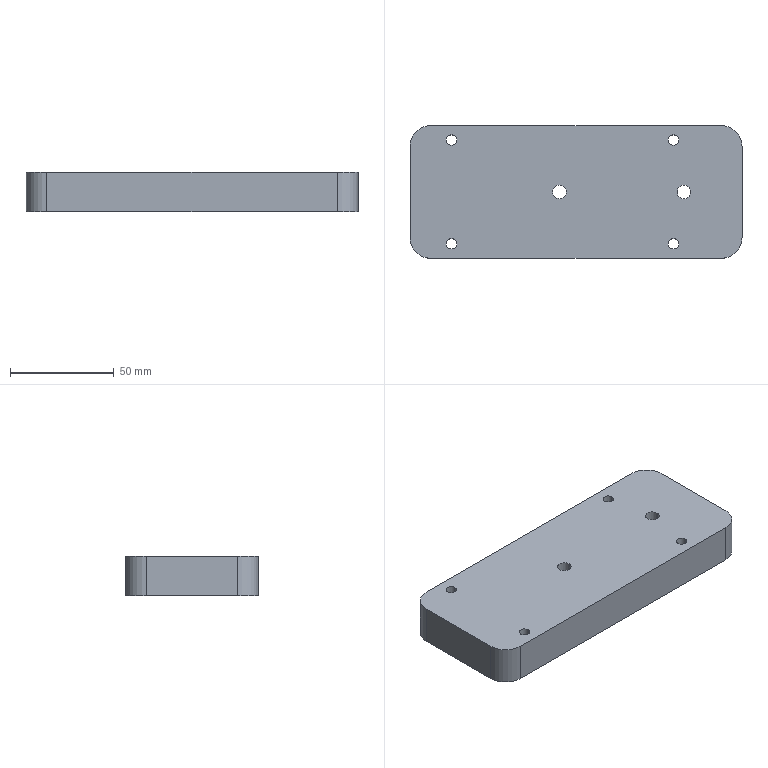Part | SolidWorks | features HoleWzd 2, Extrusion 1, Fillet 1 | 1 solid | 26 faces | box 160 x 64 x 19 mm | volume 189875 mm3 | cylinder 16 | plane 6 | cone 4 | commonest cylinder face diameters 5 x8 6.6 x4 20 x4
STEP:
#1=CARTESIAN_POINT('',(55.3,0.,3.1));
#2=VERTEX_POINT('',#1);
#3=CARTESIAN_POINT('',(48.7,0.,3.1));
#4=VERTEX_POINT('',#3);
#5=CARTESIAN_POINT('',(52.,0.,3.1));
#6=DIRECTION('',(0.,0.,-1.));
#7=DIRECTION('',(-1.,0.,0.));
#8=AXIS2_PLACEMENT_3D('',#5,#6,#7);
#9=CIRCLE('',#8,3.3);
#10=EDGE_CURVE('',#2,#4,#9,.T.);
#11=ORIENTED_EDGE('',*,*,#10,.F.);
#12=CARTESIAN_POINT('',(58.4,0.,0.));
#13=VERTEX_POINT('',#12);
#14=CARTESIAN_POINT('',(58.4,0.,0.));
#15=DIRECTION('',(0.7071,0.,-0.7071));
#16=VECTOR('',#15,1000.);
#17=LINE('',#14,#16);
#18=EDGE_CURVE('',#2,#13,#17,.T.);
#19=ORIENTED_EDGE('',*,*,#18,.T.);
#20=CARTESIAN_POINT('',(45.6,0.,0.));
#21=VERTEX_POINT('',#20);
#22=CARTESIAN_POINT('',(52.,0.,0.));
#23=DIRECTION('',(0.,0.,-1.));
#24=DIRECTION('',(-1.,0.,0.));
#25=AXIS2_PLACEMENT_3D('',#22,#23,#24);
#26=CIRCLE('',#25,6.4);
#27=EDGE_CURVE('',#13,#21,#26,.T.);
#28=ORIENTED_EDGE('',*,*,#27,.T.);
#29=CARTESIAN_POINT('',(45.6,0.,0.));
#30=DIRECTION('',(-0.7071,0.,-0.7071));
#31=VECTOR('',#30,1000.);
#32=LINE('',#29,#31);
#33=EDGE_CURVE('',#4,#21,#32,.T.);
#34=ORIENTED_EDGE('',*,*,#33,.F.);
#35=EDGE_LOOP('',(#11,#19,#28,#34));
#36=FACE_OUTER_BOUND('',#35,.T.);
#37=CARTESIAN_POINT('',(52.,0.,0.));
#38=DIRECTION('',(0.,0.,-1.));
#39=DIRECTION('',(-1.,0.,0.));
#40=AXIS2_PLACEMENT_3D('',#37,#38,#39);
#41=CONICAL_SURFACE('',#40,6.4,0.7854);
#42=ADVANCED_FACE('',(#36),#41,.F.);
#43=CARTESIAN_POINT('',(55.3,0.,19.));
#44=VERTEX_POINT('',#43);
#45=CARTESIAN_POINT('',(48.7,0.,19.));
#46=VERTEX_POINT('',#45);
#47=CARTESIAN_POINT('',(52.,0.,19.));
#48=DIRECTION('',(0.,0.,-1.));
#49=DIRECTION('',(-1.,0.,0.));
#50=AXIS2_PLACEMENT_3D('',#47,#48,#49);
#51=CIRCLE('',#50,3.3);
#52=EDGE_CURVE('',#44,#46,#51,.T.);
#53=ORIENTED_EDGE('',*,*,#52,.F.);
#54=CARTESIAN_POINT('',(55.3,0.,0.));
#55=DIRECTION('',(0.,0.,-1.));
#56=VECTOR('',#55,1000.);
#57=LINE('',#54,#56);
#58=EDGE_CURVE('',#44,#2,#57,.T.);
#59=ORIENTED_EDGE('',*,*,#58,.T.);
#60=ORIENTED_EDGE('',*,*,#10,.T.);
#61=CARTESIAN_POINT('',(48.7,0.,0.));
#62=DIRECTION('',(0.,0.,-1.));
#63=VECTOR('',#62,1000.);
#64=LINE('',#61,#63);
#65=EDGE_CURVE('',#46,#4,#64,.T.);
#66=ORIENTED_EDGE('',*,*,#65,.F.);
#67=EDGE_LOOP('',(#53,#59,#60,#66));
#68=FACE_OUTER_BOUND('',#67,.T.);
#69=CARTESIAN_POINT('',(52.,0.,0.));
#70=DIRECTION('',(0.,0.,-1.));
#71=DIRECTION('',(-1.,0.,0.));
#72=AXIS2_PLACEMENT_3D('',#69,#70,#71);
#73=CYLINDRICAL_SURFACE('',#72,3.3);
#74=ADVANCED_FACE('',(#68),#73,.F.);
#75=CARTESIAN_POINT('',(-4.7,0.,3.1));
#76=VERTEX_POINT('',#75);
#77=CARTESIAN_POINT('',(-11.3,0.,3.1));
#78=VERTEX_POINT('',#77);
#79=CARTESIAN_POINT('',(-8.,0.,3.1));
#80=DIRECTION('',(0.,0.,-1.));
#81=DIRECTION('',(-1.,0.,0.));
#82=AXIS2_PLACEMENT_3D('',#79,#80,#81);
#83=CIRCLE('',#82,3.3);
#84=EDGE_CURVE('',#76,#78,#83,.T.);
#85=ORIENTED_EDGE('',*,*,#84,.F.);
#86=CARTESIAN_POINT('',(-1.6,0.,0.));
#87=VERTEX_POINT('',#86);
#88=CARTESIAN_POINT('',(-1.6,0.,0.));
#89=DIRECTION('',(0.7071,0.,-0.7071));
#90=VECTOR('',#89,1000.);
#91=LINE('',#88,#90);
#92=EDGE_CURVE('',#76,#87,#91,.T.);
#93=ORIENTED_EDGE('',*,*,#92,.T.);
#94=CARTESIAN_POINT('',(-14.4,0.,0.));
#95=VERTEX_POINT('',#94);
#96=CARTESIAN_POINT('',(-8.,0.,0.));
#97=DIRECTION('',(0.,0.,-1.));
#98=DIRECTION('',(-1.,0.,0.));
#99=AXIS2_PLACEMENT_3D('',#96,#97,#98);
#100=CIRCLE('',#99,6.4);
#101=EDGE_CURVE('',#87,#95,#100,.T.);
#102=ORIENTED_EDGE('',*,*,#101,.T.);
#103=CARTESIAN_POINT('',(-14.4,0.,0.));
#104=DIRECTION('',(-0.7071,0.,-0.7071));
#105=VECTOR('',#104,1000.);
#106=LINE('',#103,#105);
#107=EDGE_CURVE('',#78,#95,#106,.T.);
#108=ORIENTED_EDGE('',*,*,#107,.F.);
#109=EDGE_LOOP('',(#85,#93,#102,#108));
#110=FACE_OUTER_BOUND('',#109,.T.);
#111=CARTESIAN_POINT('',(-8.,0.,0.));
#112=DIRECTION('',(0.,0.,-1.));
#113=DIRECTION('',(-1.,0.,0.));
#114=AXIS2_PLACEMENT_3D('',#111,#112,#113);
#115=CONICAL_SURFACE('',#114,6.4,0.7854);
#116=ADVANCED_FACE('',(#110),#115,.F.);
#117=CARTESIAN_POINT('',(-4.7,0.,19.));
#118=VERTEX_POINT('',#117);
#119=CARTESIAN_POINT('',(-11.3,0.,19.));
#120=VERTEX_POINT('',#119);
#121=CARTESIAN_POINT('',(-8.,0.,19.));
#122=DIRECTION('',(0.,0.,-1.));
#123=DIRECTION('',(-1.,0.,0.));
#124=AXIS2_PLACEMENT_3D('',#121,#122,#123);
#125=CIRCLE('',#124,3.3);
#126=EDGE_CURVE('',#118,#120,#125,.T.);
#127=ORIENTED_EDGE('',*,*,#126,.F.);
#128=CARTESIAN_POINT('',(-4.7,0.,0.));
#129=DIRECTION('',(0.,0.,-1.));
#130=VECTOR('',#129,1000.);
#131=LINE('',#128,#130);
#132=EDGE_CURVE('',#118,#76,#131,.T.);
#133=ORIENTED_EDGE('',*,*,#132,.T.);
#134=ORIENTED_EDGE('',*,*,#84,.T.);
#135=CARTESIAN_POINT('',(-11.3,0.,0.));
#136=DIRECTION('',(0.,0.,-1.));
#137=VECTOR('',#136,1000.);
#138=LINE('',#135,#137);
#139=EDGE_CURVE('',#120,#78,#138,.T.);
#140=ORIENTED_EDGE('',*,*,#139,.F.);
#141=EDGE_LOOP('',(#127,#133,#134,#140));
#142=FACE_OUTER_BOUND('',#141,.T.);
#143=CARTESIAN_POINT('',(-8.,0.,0.));
#144=DIRECTION('',(0.,0.,-1.));
#145=DIRECTION('',(-1.,0.,0.));
#146=AXIS2_PLACEMENT_3D('',#143,#144,#145);
#147=CYLINDRICAL_SURFACE('',#146,3.3);
#148=ADVANCED_FACE('',(#142),#147,.F.);
#149=CARTESIAN_POINT('',(-62.5,25.,0.));
#150=VERTEX_POINT('',#149);
#151=CARTESIAN_POINT('',(-57.5,25.,0.));
#152=VERTEX_POINT('',#151);
#153=CARTESIAN_POINT('',(-60.,25.,0.));
#154=DIRECTION('',(0.,0.,1.));
#155=DIRECTION('',(1.,0.,0.));
#156=AXIS2_PLACEMENT_3D('',#153,#154,#155);
#157=CIRCLE('',#156,2.5);
#158=EDGE_CURVE('',#150,#152,#157,.T.);
#159=ORIENTED_EDGE('',*,*,#158,.F.);
#160=CARTESIAN_POINT('',(-62.5,25.,19.));
#161=VERTEX_POINT('',#160);
#162=CARTESIAN_POINT('',(-62.5,25.,19.));
#163=DIRECTION('',(0.,0.,1.));
#164=VECTOR('',#163,1000.);
#165=LINE('',#162,#164);
#166=EDGE_CURVE('',#150,#161,#165,.T.);
#167=ORIENTED_EDGE('',*,*,#166,.T.);
#168=CARTESIAN_POINT('',(-57.5,25.,19.));
#169=VERTEX_POINT('',#168);
#170=CARTESIAN_POINT('',(-60.,25.,19.));
#171=DIRECTION('',(0.,0.,1.));
#172=DIRECTION('',(1.,0.,0.));
#173=AXIS2_PLACEMENT_3D('',#170,#171,#172);
#174=CIRCLE('',#173,2.5);
#175=EDGE_CURVE('',#161,#169,#174,.T.);
#176=ORIENTED_EDGE('',*,*,#175,.T.);
#177=CARTESIAN_POINT('',(-57.5,25.,19.));
#178=DIRECTION('',(0.,0.,1.));
#179=VECTOR('',#178,1000.);
#180=LINE('',#177,#179);
#181=EDGE_CURVE('',#152,#169,#180,.T.);
#182=ORIENTED_EDGE('',*,*,#181,.F.);
#183=EDGE_LOOP('',(#159,#167,#176,#182));
#184=FACE_OUTER_BOUND('',#183,.T.);
#185=CARTESIAN_POINT('',(-60.,25.,19.));
#186=DIRECTION('',(0.,0.,1.));
#187=DIRECTION('',(1.,0.,0.));
#188=AXIS2_PLACEMENT_3D('',#185,#186,#187);
#189=CYLINDRICAL_SURFACE('',#188,2.5);
#190=ADVANCED_FACE('',(#184),#189,.F.);
#191=CARTESIAN_POINT('',(-62.5,-25.,0.));
#192=VERTEX_POINT('',#191);
#193=CARTESIAN_POINT('',(-57.5,-25.,0.));
#194=VERTEX_POINT('',#193);
#195=CARTESIAN_POINT('',(-60.,-25.,0.));
#196=DIRECTION('',(0.,0.,1.));
#197=DIRECTION('',(1.,0.,0.));
#198=AXIS2_PLACEMENT_3D('',#195,#196,#197);
#199=CIRCLE('',#198,2.5);
#200=EDGE_CURVE('',#192,#194,#199,.T.);
#201=ORIENTED_EDGE('',*,*,#200,.F.);
#202=CARTESIAN_POINT('',(-62.5,-25.,19.));
#203=VERTEX_POINT('',#202);
#204=CARTESIAN_POINT('',(-62.5,-25.,19.));
#205=DIRECTION('',(0.,0.,1.));
#206=VECTOR('',#205,1000.);
#207=LINE('',#204,#206);
#208=EDGE_CURVE('',#192,#203,#207,.T.);
#209=ORIENTED_EDGE('',*,*,#208,.T.);
#210=CARTESIAN_POINT('',(-57.5,-25.,19.));
#211=VERTEX_POINT('',#210);
#212=CARTESIAN_POINT('',(-60.,-25.,19.));
#213=DIRECTION('',(0.,0.,1.));
#214=DIRECTION('',(1.,0.,0.));
#215=AXIS2_PLACEMENT_3D('',#212,#213,#214);
#216=CIRCLE('',#215,2.5);
#217=EDGE_CURVE('',#203,#211,#216,.T.);
#218=ORIENTED_EDGE('',*,*,#217,.T.);
#219=CARTESIAN_POINT('',(-57.5,-25.,19.));
#220=DIRECTION('',(0.,0.,1.));
#221=VECTOR('',#220,1000.);
#222=LINE('',#219,#221);
#223=EDGE_CURVE('',#194,#211,#222,.T.);
#224=ORIENTED_EDGE('',*,*,#223,.F.);
#225=EDGE_LOOP('',(#201,#209,#218,#224));
#226=FACE_OUTER_BOUND('',#225,.T.);
#227=CARTESIAN_POINT('',(-60.,-25.,19.));
#228=DIRECTION('',(0.,0.,1.));
#229=DIRECTION('',(1.,0.,0.));
#230=AXIS2_PLACEMENT_3D('',#227,#228,#229);
#231=CYLINDRICAL_SURFACE('',#230,2.5);
#232=ADVANCED_FACE('',(#226),#231,.F.);
#233=CARTESIAN_POINT('',(44.5,25.,0.));
#234=VERTEX_POINT('',#233);
#235=CARTESIAN_POINT('',(49.5,25.,0.));
#236=VERTEX_POINT('',#235);
#237=CARTESIAN_POINT('',(47.,25.,0.));
#238=DIRECTION('',(0.,0.,1.));
#239=DIRECTION('',(1.,0.,0.));
#240=AXIS2_PLACEMENT_3D('',#237,#238,#239);
#241=CIRCLE('',#240,2.5);
#242=EDGE_CURVE('',#234,#236,#241,.T.);
#243=ORIENTED_EDGE('',*,*,#242,.F.);
#244=CARTESIAN_POINT('',(44.5,25.,19.));
#245=VERTEX_POINT('',#244);
#246=CARTESIAN_POINT('',(44.5,25.,19.));
#247=DIRECTION('',(0.,0.,1.));
#248=VECTOR('',#247,1000.);
#249=LINE('',#246,#248);
#250=EDGE_CURVE('',#234,#245,#249,.T.);
#251=ORIENTED_EDGE('',*,*,#250,.T.);
#252=CARTESIAN_POINT('',(49.5,25.,19.));
#253=VERTEX_POINT('',#252);
#254=CARTESIAN_POINT('',(47.,25.,19.));
#255=DIRECTION('',(0.,0.,1.));
#256=DIRECTION('',(1.,0.,0.));
#257=AXIS2_PLACEMENT_3D('',#254,#255,#256);
#258=CIRCLE('',#257,2.5);
#259=EDGE_CURVE('',#245,#253,#258,.T.);
#260=ORIENTED_EDGE('',*,*,#259,.T.);
#261=CARTESIAN_POINT('',(49.5,25.,19.));
#262=DIRECTION('',(0.,0.,1.));
#263=VECTOR('',#262,1000.);
#264=LINE('',#261,#263);
#265=EDGE_CURVE('',#236,#253,#264,.T.);
#266=ORIENTED_EDGE('',*,*,#265,.F.);
#267=EDGE_LOOP('',(#243,#251,#260,#266));
#268=FACE_OUTER_BOUND('',#267,.T.);
#269=CARTESIAN_POINT('',(47.,25.,19.));
#270=DIRECTION('',(0.,0.,1.));
#271=DIRECTION('',(1.,0.,0.));
#272=AXIS2_PLACEMENT_3D('',#269,#270,#271);
#273=CYLINDRICAL_SURFACE('',#272,2.5);
#274=ADVANCED_FACE('',(#268),#273,.F.);
#275=CARTESIAN_POINT('',(44.5,-25.,0.));
#276=VERTEX_POINT('',#275);
#277=CARTESIAN_POINT('',(49.5,-25.,0.));
#278=VERTEX_POINT('',#277);
#279=CARTESIAN_POINT('',(47.,-25.,0.));
#280=DIRECTION('',(0.,0.,1.));
#281=DIRECTION('',(1.,0.,0.));
#282=AXIS2_PLACEMENT_3D('',#279,#280,#281);
#283=CIRCLE('',#282,2.5);
#284=EDGE_CURVE('',#276,#278,#283,.T.);
#285=ORIENTED_EDGE('',*,*,#284,.F.);
#286=CARTESIAN_POINT('',(44.5,-25.,19.));
#287=VERTEX_POINT('',#286);
#288=CARTESIAN_POINT('',(44.5,-25.,19.));
#289=DIRECTION('',(0.,0.,1.));
#290=VECTOR('',#289,1000.);
#291=LINE('',#288,#290);
#292=EDGE_CURVE('',#276,#287,#291,.T.);
#293=ORIENTED_EDGE('',*,*,#292,.T.);
#294=CARTESIAN_POINT('',(49.5,-25.,19.));
#295=VERTEX_POINT('',#294);
#296=CARTESIAN_POINT('',(47.,-25.,19.));
#297=DIRECTION('',(0.,0.,1.));
#298=DIRECTION('',(1.,0.,0.));
#299=AXIS2_PLACEMENT_3D('',#296,#297,#298);
#300=CIRCLE('',#299,2.5);
#301=EDGE_CURVE('',#287,#295,#300,.T.);
#302=ORIENTED_EDGE('',*,*,#301,.T.);
#303=CARTESIAN_POINT('',(49.5,-25.,19.));
#304=DIRECTION('',(0.,0.,1.));
#305=VECTOR('',#304,1000.);
#306=LINE('',#303,#305);
#307=EDGE_CURVE('',#278,#295,#306,.T.);
#308=ORIENTED_EDGE('',*,*,#307,.F.);
#309=EDGE_LOOP('',(#285,#293,#302,#308));
#310=FACE_OUTER_BOUND('',#309,.T.);
#311=CARTESIAN_POINT('',(47.,-25.,19.));
#312=DIRECTION('',(0.,0.,1.));
#313=DIRECTION('',(1.,0.,0.));
#314=AXIS2_PLACEMENT_3D('',#311,#312,#313);
#315=CYLINDRICAL_SURFACE('',#314,2.5);
#316=ADVANCED_FACE('',(#310),#315,.F.);
#317=CARTESIAN_POINT('',(80.,-22.,0.));
#318=VERTEX_POINT('',#317);
#319=CARTESIAN_POINT('',(80.,22.,0.));
#320=VERTEX_POINT('',#319);
#321=CARTESIAN_POINT('',(80.,32.,0.));
#322=DIRECTION('',(0.,1.,0.));
#323=VECTOR('',#322,1000.);
#324=LINE('',#321,#323);
#325=EDGE_CURVE('',#318,#320,#324,.T.);
#326=ORIENTED_EDGE('',*,*,#325,.T.);
#327=CARTESIAN_POINT('',(80.,22.,19.));
#328=VERTEX_POINT('',#327);
#329=CARTESIAN_POINT('',(80.,22.,19.));
#330=DIRECTION('',(0.,0.,1.));
#331=VECTOR('',#330,1000.);
#332=LINE('',#329,#331);
#333=EDGE_CURVE('',#320,#328,#332,.T.);
#334=ORIENTED_EDGE('',*,*,#333,.T.);
#335=CARTESIAN_POINT('',(80.,-22.,19.));
#336=VERTEX_POINT('',#335);
#337=CARTESIAN_POINT('',(80.,32.,19.));
#338=DIRECTION('',(0.,1.,0.));
#339=VECTOR('',#338,1000.);
#340=LINE('',#337,#339);
#341=EDGE_CURVE('',#336,#328,#340,.T.);
#342=ORIENTED_EDGE('',*,*,#341,.F.);
#343=CARTESIAN_POINT('',(80.,-22.,19.));
#344=DIRECTION('',(0.,0.,-1.));
#345=VECTOR('',#344,1000.);
#346=LINE('',#343,#345);
#347=EDGE_CURVE('',#336,#318,#346,.T.);
#348=ORIENTED_EDGE('',*,*,#347,.T.);
#349=EDGE_LOOP('',(#326,#334,#342,#348));
#350=FACE_OUTER_BOUND('',#349,.T.);
#351=CARTESIAN_POINT('',(80.,32.,19.));
#352=DIRECTION('',(-1.,0.,0.));
#353=DIRECTION('',(0.,0.,1.));
#354=AXIS2_PLACEMENT_3D('',#351,#352,#353);
#355=PLANE('',#354);
#356=ADVANCED_FACE('',(#350),#355,.F.);
#357=CARTESIAN_POINT('',(70.,32.,19.));
#358=VERTEX_POINT('',#357);
#359=CARTESIAN_POINT('',(-70.,32.,19.));
#360=VERTEX_POINT('',#359);
#361=CARTESIAN_POINT('',(-80.,32.,19.));
#362=DIRECTION('',(-1.,0.,0.));
#363=VECTOR('',#362,1000.);
#364=LINE('',#361,#363);
#365=EDGE_CURVE('',#358,#360,#364,.T.);
#366=ORIENTED_EDGE('',*,*,#365,.F.);
#367=CARTESIAN_POINT('',(70.,32.,0.));
#368=VERTEX_POINT('',#367);
#369=CARTESIAN_POINT('',(70.,32.,19.));
#370=DIRECTION('',(0.,0.,-1.));
#371=VECTOR('',#370,1000.);
#372=LINE('',#369,#371);
#373=EDGE_CURVE('',#358,#368,#372,.T.);
#374=ORIENTED_EDGE('',*,*,#373,.T.);
#375=CARTESIAN_POINT('',(-70.,32.,0.));
#376=VERTEX_POINT('',#375);
#377=CARTESIAN_POINT('',(-80.,32.,0.));
#378=DIRECTION('',(-1.,0.,0.));
#379=VECTOR('',#378,1000.);
#380=LINE('',#377,#379);
#381=EDGE_CURVE('',#368,#376,#380,.T.);
#382=ORIENTED_EDGE('',*,*,#381,.T.);
#383=CARTESIAN_POINT('',(-70.,32.,19.));
#384=DIRECTION('',(0.,0.,1.));
#385=VECTOR('',#384,1000.);
#386=LINE('',#383,#385);
#387=EDGE_CURVE('',#376,#360,#386,.T.);
#388=ORIENTED_EDGE('',*,*,#387,.T.);
#389=EDGE_LOOP('',(#366,#374,#382,#388));
#390=FACE_OUTER_BOUND('',#389,.T.);
#391=CARTESIAN_POINT('',(-80.,32.,19.));
#392=DIRECTION('',(0.,-1.,0.));
#393=DIRECTION('',(0.,0.,-1.));
#394=AXIS2_PLACEMENT_3D('',#391,#392,#393);
#395=PLANE('',#394);
#396=ADVANCED_FACE('',(#390),#395,.F.);
#397=CARTESIAN_POINT('',(-80.,22.,19.));
#398=VERTEX_POINT('',#397);
#399=CARTESIAN_POINT('',(-80.,-22.,19.));
#400=VERTEX_POINT('',#399);
#401=CARTESIAN_POINT('',(-80.,32.,19.));
#402=DIRECTION('',(0.,-1.,0.));
#403=VECTOR('',#402,1000.);
#404=LINE('',#401,#403);
#405=EDGE_CURVE('',#398,#400,#404,.T.);
#406=ORIENTED_EDGE('',*,*,#405,.F.);
#407=CARTESIAN_POINT('',(-80.,22.,0.));
#408=VERTEX_POINT('',#407);
#409=CARTESIAN_POINT('',(-80.,22.,19.));
#410=DIRECTION('',(0.,0.,-1.));
#411=VECTOR('',#410,1000.);
#412=LINE('',#409,#411);
#413=EDGE_CURVE('',#398,#408,#412,.T.);
#414=ORIENTED_EDGE('',*,*,#413,.T.);
#415=CARTESIAN_POINT('',(-80.,-22.,0.));
#416=VERTEX_POINT('',#415);
#417=CARTESIAN_POINT('',(-80.,32.,0.));
#418=DIRECTION('',(0.,-1.,0.));
#419=VECTOR('',#418,1000.);
#420=LINE('',#417,#419);
#421=EDGE_CURVE('',#408,#416,#420,.T.);
#422=ORIENTED_EDGE('',*,*,#421,.T.);
#423=CARTESIAN_POINT('',(-80.,-22.,19.));
#424=DIRECTION('',(0.,0.,1.));
#425=VECTOR('',#424,1000.);
#426=LINE('',#423,#425);
#427=EDGE_CURVE('',#416,#400,#426,.T.);
#428=ORIENTED_EDGE('',*,*,#427,.T.);
#429=EDGE_LOOP('',(#406,#414,#422,#428));
#430=FACE_OUTER_BOUND('',#429,.T.);
#431=CARTESIAN_POINT('',(-80.,32.,19.));
#432=DIRECTION('',(1.,0.,0.));
#433=DIRECTION('',(0.,1.,0.));
#434=AXIS2_PLACEMENT_3D('',#431,#432,#433);
#435=PLANE('',#434);
#436=ADVANCED_FACE('',(#430),#435,.F.);
#437=CARTESIAN_POINT('',(-70.,-32.,0.));
#438=VERTEX_POINT('',#437);
#439=CARTESIAN_POINT('',(70.,-32.,0.));
#440=VERTEX_POINT('',#439);
#441=CARTESIAN_POINT('',(-80.,-32.,0.));
#442=DIRECTION('',(1.,0.,0.));
#443=VECTOR('',#442,1000.);
#444=LINE('',#441,#443);
#445=EDGE_CURVE('',#438,#440,#444,.T.);
#446=ORIENTED_EDGE('',*,*,#445,.T.);
#447=CARTESIAN_POINT('',(70.,-32.,19.));
#448=VERTEX_POINT('',#447);
#449=CARTESIAN_POINT('',(70.,-32.,19.));
#450=DIRECTION('',(0.,0.,1.));
#451=VECTOR('',#450,1000.);
#452=LINE('',#449,#451);
#453=EDGE_CURVE('',#440,#448,#452,.T.);
#454=ORIENTED_EDGE('',*,*,#453,.T.);
#455=CARTESIAN_POINT('',(-70.,-32.,19.));
#456=VERTEX_POINT('',#455);
#457=CARTESIAN_POINT('',(-80.,-32.,19.));
#458=DIRECTION('',(1.,0.,0.));
#459=VECTOR('',#458,1000.);
#460=LINE('',#457,#459);
#461=EDGE_CURVE('',#456,#448,#460,.T.);
#462=ORIENTED_EDGE('',*,*,#461,.F.);
#463=CARTESIAN_POINT('',(-70.,-32.,19.));
#464=DIRECTION('',(0.,0.,-1.));
#465=VECTOR('',#464,1000.);
#466=LINE('',#463,#465);
#467=EDGE_CURVE('',#456,#438,#466,.T.);
#468=ORIENTED_EDGE('',*,*,#467,.T.);
#469=EDGE_LOOP('',(#446,#454,#462,#468));
#470=FACE_OUTER_BOUND('',#469,.T.);
#471=CARTESIAN_POINT('',(-80.,-32.,19.));
#472=DIRECTION('',(0.,1.,0.));
#473=DIRECTION('',(0.,0.,1.));
#474=AXIS2_PLACEMENT_3D('',#471,#472,#473);
#475=PLANE('',#474);
#476=ADVANCED_FACE('',(#470),#475,.F.);
#477=CARTESIAN_POINT('',(52.,0.,19.));
#478=DIRECTION('',(0.,0.,-1.));
#479=DIRECTION('',(-1.,0.,0.));
#480=AXIS2_PLACEMENT_3D('',#477,#478,#479);
#481=CIRCLE('',#480,3.3);
#482=EDGE_CURVE('',#46,#44,#481,.T.);
#483=ORIENTED_EDGE('',*,*,#482,.T.);
#484=ORIENTED_EDGE('',*,*,#52,.T.);
#485=EDGE_LOOP('',(#483,#484));
#486=FACE_BOUND('',#485,.T.);
#487=CARTESIAN_POINT('',(-8.,0.,19.));
#488=DIRECTION('',(0.,0.,-1.));
#489=DIRECTION('',(-1.,0.,0.));
#490=AXIS2_PLACEMENT_3D('',#487,#488,#489);
#491=CIRCLE('',#490,3.3);
#492=EDGE_CURVE('',#120,#118,#491,.T.);
#493=ORIENTED_EDGE('',*,*,#492,.T.);
#494=ORIENTED_EDGE('',*,*,#126,.T.);
#495=EDGE_LOOP('',(#493,#494));
#496=FACE_BOUND('',#495,.T.);
#497=CARTESIAN_POINT('',(-60.,25.,19.));
#498=DIRECTION('',(0.,0.,1.));
#499=DIRECTION('',(1.,0.,0.));
#500=AXIS2_PLACEMENT_3D('',#497,#498,#499);
#501=CIRCLE('',#500,2.5);
#502=EDGE_CURVE('',#169,#161,#501,.T.);
#503=ORIENTED_EDGE('',*,*,#502,.F.);
#504=ORIENTED_EDGE('',*,*,#175,.F.);
#505=EDGE_LOOP('',(#503,#504));
#506=FACE_BOUND('',#505,.T.);
#507=CARTESIAN_POINT('',(-60.,-25.,19.));
#508=DIRECTION('',(0.,0.,1.));
#509=DIRECTION('',(1.,0.,0.));
#510=AXIS2_PLACEMENT_3D('',#507,#508,#509);
#511=CIRCLE('',#510,2.5);
#512=EDGE_CURVE('',#211,#203,#511,.T.);
#513=ORIENTED_EDGE('',*,*,#512,.F.);
#514=ORIENTED_EDGE('',*,*,#217,.F.);
#515=EDGE_LOOP('',(#513,#514));
#516=FACE_BOUND('',#515,.T.);
#517=CARTESIAN_POINT('',(47.,25.,19.));
#518=DIRECTION('',(0.,0.,1.));
#519=DIRECTION('',(1.,0.,0.));
#520=AXIS2_PLACEMENT_3D('',#517,#518,#519);
#521=CIRCLE('',#520,2.5);
#522=EDGE_CURVE('',#253,#245,#521,.T.);
#523=ORIENTED_EDGE('',*,*,#522,.F.);
#524=ORIENTED_EDGE('',*,*,#259,.F.);
#525=EDGE_LOOP('',(#523,#524));
#526=FACE_BOUND('',#525,.T.);
#527=CARTESIAN_POINT('',(47.,-25.,19.));
#528=DIRECTION('',(0.,0.,1.));
#529=DIRECTION('',(1.,0.,0.));
#530=AXIS2_PLACEMENT_3D('',#527,#528,#529);
#531=CIRCLE('',#530,2.5);
#532=EDGE_CURVE('',#295,#287,#531,.T.);
#533=ORIENTED_EDGE('',*,*,#532,.F.);
#534=ORIENTED_EDGE('',*,*,#301,.F.);
#535=EDGE_LOOP('',(#533,#534));
#536=FACE_BOUND('',#535,.T.);
#537=ORIENTED_EDGE('',*,*,#341,.T.);
#538=CARTESIAN_POINT('',(70.,22.,19.));
#539=DIRECTION('',(0.,0.,1.));
#540=DIRECTION('',(1.,0.,0.));
#541=AXIS2_PLACEMENT_3D('',#538,#539,#540);
#542=CIRCLE('',#541,10.);
#543=EDGE_CURVE('',#328,#358,#542,.T.);
#544=ORIENTED_EDGE('',*,*,#543,.T.);
#545=ORIENTED_EDGE('',*,*,#365,.T.);
#546=CARTESIAN_POINT('',(-70.,22.,19.));
#547=DIRECTION('',(0.,0.,1.));
#548=DIRECTION('',(1.,0.,0.));
#549=AXIS2_PLACEMENT_3D('',#546,#547,#548);
#550=CIRCLE('',#549,10.);
#551=EDGE_CURVE('',#360,#398,#550,.T.);
#552=ORIENTED_EDGE('',*,*,#551,.T.);
#553=ORIENTED_EDGE('',*,*,#405,.T.);
#554=CARTESIAN_POINT('',(-70.,-22.,19.));
#555=DIRECTION('',(0.,0.,1.));
#556=DIRECTION('',(1.,0.,0.));
#557=AXIS2_PLACEMENT_3D('',#554,#555,#556);
#558=CIRCLE('',#557,10.);
#559=EDGE_CURVE('',#400,#456,#558,.T.);
#560=ORIENTED_EDGE('',*,*,#559,.T.);
#561=ORIENTED_EDGE('',*,*,#461,.T.);
#562=CARTESIAN_POINT('',(70.,-22.,19.));
#563=DIRECTION('',(0.,0.,1.));
#564=DIRECTION('',(1.,0.,0.));
#565=AXIS2_PLACEMENT_3D('',#562,#563,#564);
#566=CIRCLE('',#565,10.);
#567=EDGE_CURVE('',#448,#336,#566,.T.);
#568=ORIENTED_EDGE('',*,*,#567,.T.);
#569=EDGE_LOOP('',(#537,#544,#545,#552,#553,#560,#561,#568));
#570=FACE_OUTER_BOUND('',#569,.T.);
#571=CARTESIAN_POINT('',(0.,0.,19.));
#572=DIRECTION('',(0.,0.,1.));
#573=DIRECTION('',(1.,0.,0.));
#574=AXIS2_PLACEMENT_3D('',#571,#572,#573);
#575=PLANE('',#574);
#576=ADVANCED_FACE('',(#486,#496,#506,#516,#526,#536,#570),#575,.T.);
#577=CARTESIAN_POINT('',(52.,0.,0.));
#578=DIRECTION('',(0.,0.,-1.));
#579=DIRECTION('',(-1.,0.,0.));
#580=AXIS2_PLACEMENT_3D('',#577,#578,#579);
#581=CIRCLE('',#580,6.4);
#582=EDGE_CURVE('',#21,#13,#581,.T.);
#583=ORIENTED_EDGE('',*,*,#582,.F.);
#584=ORIENTED_EDGE('',*,*,#27,.F.);
#585=EDGE_LOOP('',(#583,#584));
#586=FACE_BOUND('',#585,.T.);
#587=CARTESIAN_POINT('',(-8.,0.,0.));
#588=DIRECTION('',(0.,0.,-1.));
#589=DIRECTION('',(-1.,0.,0.));
#590=AXIS2_PLACEMENT_3D('',#587,#588,#589);
#591=CIRCLE('',#590,6.4);
#592=EDGE_CURVE('',#95,#87,#591,.T.);
#593=ORIENTED_EDGE('',*,*,#592,.F.);
#594=ORIENTED_EDGE('',*,*,#101,.F.);
#595=EDGE_LOOP('',(#593,#594));
#596=FACE_BOUND('',#595,.T.);
#597=CARTESIAN_POINT('',(-60.,25.,0.));
#598=DIRECTION('',(0.,0.,1.));
#599=DIRECTION('',(1.,0.,0.));
#600=AXIS2_PLACEMENT_3D('',#597,#598,#599);
#601=CIRCLE('',#600,2.5);
#602=EDGE_CURVE('',#152,#150,#601,.T.);
#603=ORIENTED_EDGE('',*,*,#602,.T.);
#604=ORIENTED_EDGE('',*,*,#158,.T.);
#605=EDGE_LOOP('',(#603,#604));
#606=FACE_BOUND('',#605,.T.);
#607=CARTESIAN_POINT('',(-60.,-25.,0.));
#608=DIRECTION('',(0.,0.,1.));
#609=DIRECTION('',(1.,0.,0.));
#610=AXIS2_PLACEMENT_3D('',#607,#608,#609);
#611=CIRCLE('',#610,2.5);
#612=EDGE_CURVE('',#194,#192,#611,.T.);
#613=ORIENTED_EDGE('',*,*,#612,.T.);
#614=ORIENTED_EDGE('',*,*,#200,.T.);
#615=EDGE_LOOP('',(#613,#614));
#616=FACE_BOUND('',#615,.T.);
#617=CARTESIAN_POINT('',(47.,25.,0.));
#618=DIRECTION('',(0.,0.,1.));
#619=DIRECTION('',(1.,0.,0.));
#620=AXIS2_PLACEMENT_3D('',#617,#618,#619);
#621=CIRCLE('',#620,2.5);
#622=EDGE_CURVE('',#236,#234,#621,.T.);
#623=ORIENTED_EDGE('',*,*,#622,.T.);
#624=ORIENTED_EDGE('',*,*,#242,.T.);
#625=EDGE_LOOP('',(#623,#624));
#626=FACE_BOUND('',#625,.T.);
#627=CARTESIAN_POINT('',(47.,-25.,0.));
#628=DIRECTION('',(0.,0.,1.));
#629=DIRECTION('',(1.,0.,0.));
#630=AXIS2_PLACEMENT_3D('',#627,#628,#629);
#631=CIRCLE('',#630,2.5);
#632=EDGE_CURVE('',#278,#276,#631,.T.);
#633=ORIENTED_EDGE('',*,*,#632,.T.);
#634=ORIENTED_EDGE('',*,*,#284,.T.);
#635=EDGE_LOOP('',(#633,#634));
#636=FACE_BOUND('',#635,.T.);
#637=ORIENTED_EDGE('',*,*,#381,.F.);
#638=CARTESIAN_POINT('',(70.,22.,0.));
#639=DIRECTION('',(0.,0.,-1.));
#640=DIRECTION('',(1.,0.,0.));
#641=AXIS2_PLACEMENT_3D('',#638,#639,#640);
#642=CIRCLE('',#641,10.);
#643=EDGE_CURVE('',#368,#320,#642,.T.);
#644=ORIENTED_EDGE('',*,*,#643,.T.);
#645=ORIENTED_EDGE('',*,*,#325,.F.);
#646=CARTESIAN_POINT('',(70.,-22.,0.));
#647=DIRECTION('',(0.,0.,-1.));
#648=DIRECTION('',(1.,0.,0.));
#649=AXIS2_PLACEMENT_3D('',#646,#647,#648);
#650=CIRCLE('',#649,10.);
#651=EDGE_CURVE('',#318,#440,#650,.T.);
#652=ORIENTED_EDGE('',*,*,#651,.T.);
#653=ORIENTED_EDGE('',*,*,#445,.F.);
#654=CARTESIAN_POINT('',(-70.,-22.,0.));
#655=DIRECTION('',(0.,0.,-1.));
#656=DIRECTION('',(1.,0.,0.));
#657=AXIS2_PLACEMENT_3D('',#654,#655,#656);
#658=CIRCLE('',#657,10.);
#659=EDGE_CURVE('',#438,#416,#658,.T.);
#660=ORIENTED_EDGE('',*,*,#659,.T.);
#661=ORIENTED_EDGE('',*,*,#421,.F.);
#662=CARTESIAN_POINT('',(-70.,22.,0.));
#663=DIRECTION('',(0.,0.,-1.));
#664=DIRECTION('',(1.,0.,0.));
#665=AXIS2_PLACEMENT_3D('',#662,#663,#664);
#666=CIRCLE('',#665,10.);
#667=EDGE_CURVE('',#408,#376,#666,.T.);
#668=ORIENTED_EDGE('',*,*,#667,.T.);
#669=EDGE_LOOP('',(#637,#644,#645,#652,#653,#660,#661,#668));
#670=FACE_OUTER_BOUND('',#669,.T.);
#671=CARTESIAN_POINT('',(0.,0.,0.));
#672=DIRECTION('',(0.,0.,1.));
#673=DIRECTION('',(1.,0.,0.));
#674=AXIS2_PLACEMENT_3D('',#671,#672,#673);
#675=PLANE('',#674);
#676=ADVANCED_FACE('',(#586,#596,#606,#616,#626,#636,#670),#675,.F.);
#677=ORIENTED_EDGE('',*,*,#543,.F.);
#678=ORIENTED_EDGE('',*,*,#333,.F.);
#679=ORIENTED_EDGE('',*,*,#643,.F.);
#680=ORIENTED_EDGE('',*,*,#373,.F.);
#681=EDGE_LOOP('',(#677,#678,#679,#680));
#682=FACE_OUTER_BOUND('',#681,.T.);
#683=CARTESIAN_POINT('',(70.,22.,19.));
#684=DIRECTION('',(0.,0.,-1.));
#685=DIRECTION('',(-1.,0.,0.));
#686=AXIS2_PLACEMENT_3D('',#683,#684,#685);
#687=CYLINDRICAL_SURFACE('',#686,10.);
#688=ADVANCED_FACE('',(#682),#687,.T.);
#689=ORIENTED_EDGE('',*,*,#567,.F.);
#690=ORIENTED_EDGE('',*,*,#453,.F.);
#691=ORIENTED_EDGE('',*,*,#651,.F.);
#692=ORIENTED_EDGE('',*,*,#347,.F.);
#693=EDGE_LOOP('',(#689,#690,#691,#692));
#694=FACE_OUTER_BOUND('',#693,.T.);
#695=CARTESIAN_POINT('',(70.,-22.,19.));
#696=DIRECTION('',(0.,0.,-1.));
#697=DIRECTION('',(-1.,0.,0.));
#698=AXIS2_PLACEMENT_3D('',#695,#696,#697);
#699=CYLINDRICAL_SURFACE('',#698,10.);
#700=ADVANCED_FACE('',(#694),#699,.T.);
#701=ORIENTED_EDGE('',*,*,#551,.F.);
#702=ORIENTED_EDGE('',*,*,#387,.F.);
#703=ORIENTED_EDGE('',*,*,#667,.F.);
#704=ORIENTED_EDGE('',*,*,#413,.F.);
#705=EDGE_LOOP('',(#701,#702,#703,#704));
#706=FACE_OUTER_BOUND('',#705,.T.);
#707=CARTESIAN_POINT('',(-70.,22.,19.));
#708=DIRECTION('',(0.,0.,-1.));
#709=DIRECTION('',(-1.,0.,0.));
#710=AXIS2_PLACEMENT_3D('',#707,#708,#709);
#711=CYLINDRICAL_SURFACE('',#710,10.);
#712=ADVANCED_FACE('',(#706),#711,.T.);
#713=ORIENTED_EDGE('',*,*,#559,.F.);
#714=ORIENTED_EDGE('',*,*,#427,.F.);
#715=ORIENTED_EDGE('',*,*,#659,.F.);
#716=ORIENTED_EDGE('',*,*,#467,.F.);
#717=EDGE_LOOP('',(#713,#714,#715,#716));
#718=FACE_OUTER_BOUND('',#717,.T.);
#719=CARTESIAN_POINT('',(-70.,-22.,19.));
#720=DIRECTION('',(0.,0.,-1.));
#721=DIRECTION('',(-1.,0.,0.));
#722=AXIS2_PLACEMENT_3D('',#719,#720,#721);
#723=CYLINDRICAL_SURFACE('',#722,10.);
#724=ADVANCED_FACE('',(#718),#723,.T.);
#725=ORIENTED_EDGE('',*,*,#292,.F.);
#726=ORIENTED_EDGE('',*,*,#632,.F.);
#727=ORIENTED_EDGE('',*,*,#307,.T.);
#728=ORIENTED_EDGE('',*,*,#532,.T.);
#729=EDGE_LOOP('',(#725,#726,#727,#728));
#730=FACE_OUTER_BOUND('',#729,.T.);
#731=CARTESIAN_POINT('',(47.,-25.,19.));
#732=DIRECTION('',(0.,0.,1.));
#733=DIRECTION('',(1.,0.,0.));
#734=AXIS2_PLACEMENT_3D('',#731,#732,#733);
#735=CYLINDRICAL_SURFACE('',#734,2.5);
#736=ADVANCED_FACE('',(#730),#735,.F.);
#737=ORIENTED_EDGE('',*,*,#250,.F.);
#738=ORIENTED_EDGE('',*,*,#622,.F.);
#739=ORIENTED_EDGE('',*,*,#265,.T.);
#740=ORIENTED_EDGE('',*,*,#522,.T.);
#741=EDGE_LOOP('',(#737,#738,#739,#740));
#742=FACE_OUTER_BOUND('',#741,.T.);
#743=CARTESIAN_POINT('',(47.,25.,19.));
#744=DIRECTION('',(0.,0.,1.));
#745=DIRECTION('',(1.,0.,0.));
#746=AXIS2_PLACEMENT_3D('',#743,#744,#745);
#747=CYLINDRICAL_SURFACE('',#746,2.5);
#748=ADVANCED_FACE('',(#742),#747,.F.);
#749=ORIENTED_EDGE('',*,*,#208,.F.);
#750=ORIENTED_EDGE('',*,*,#612,.F.);
#751=ORIENTED_EDGE('',*,*,#223,.T.);
#752=ORIENTED_EDGE('',*,*,#512,.T.);
#753=EDGE_LOOP('',(#749,#750,#751,#752));
#754=FACE_OUTER_BOUND('',#753,.T.);
#755=CARTESIAN_POINT('',(-60.,-25.,19.));
#756=DIRECTION('',(0.,0.,1.));
#757=DIRECTION('',(1.,0.,0.));
#758=AXIS2_PLACEMENT_3D('',#755,#756,#757);
#759=CYLINDRICAL_SURFACE('',#758,2.5);
#760=ADVANCED_FACE('',(#754),#759,.F.);
#761=ORIENTED_EDGE('',*,*,#166,.F.);
#762=ORIENTED_EDGE('',*,*,#602,.F.);
#763=ORIENTED_EDGE('',*,*,#181,.T.);
#764=ORIENTED_EDGE('',*,*,#502,.T.);
#765=EDGE_LOOP('',(#761,#762,#763,#764));
#766=FACE_OUTER_BOUND('',#765,.T.);
#767=CARTESIAN_POINT('',(-60.,25.,19.));
#768=DIRECTION('',(0.,0.,1.));
#769=DIRECTION('',(1.,0.,0.));
#770=AXIS2_PLACEMENT_3D('',#767,#768,#769);
#771=CYLINDRICAL_SURFACE('',#770,2.5);
#772=ADVANCED_FACE('',(#766),#771,.F.);
#773=ORIENTED_EDGE('',*,*,#132,.F.);
#774=ORIENTED_EDGE('',*,*,#492,.F.);
#775=ORIENTED_EDGE('',*,*,#139,.T.);
#776=CARTESIAN_POINT('',(-8.,0.,3.1));
#777=DIRECTION('',(0.,0.,-1.));
#778=DIRECTION('',(-1.,0.,0.));
#779=AXIS2_PLACEMENT_3D('',#776,#777,#778);
#780=CIRCLE('',#779,3.3);
#781=EDGE_CURVE('',#78,#76,#780,.T.);
#782=ORIENTED_EDGE('',*,*,#781,.T.);
#783=EDGE_LOOP('',(#773,#774,#775,#782));
#784=FACE_OUTER_BOUND('',#783,.T.);
#785=CARTESIAN_POINT('',(-8.,0.,0.));
#786=DIRECTION('',(0.,0.,-1.));
#787=DIRECTION('',(-1.,0.,0.));
#788=AXIS2_PLACEMENT_3D('',#785,#786,#787);
#789=CYLINDRICAL_SURFACE('',#788,3.3);
#790=ADVANCED_FACE('',(#784),#789,.F.);
#791=ORIENTED_EDGE('',*,*,#92,.F.);
#792=ORIENTED_EDGE('',*,*,#781,.F.);
#793=ORIENTED_EDGE('',*,*,#107,.T.);
#794=ORIENTED_EDGE('',*,*,#592,.T.);
#795=EDGE_LOOP('',(#791,#792,#793,#794));
#796=FACE_OUTER_BOUND('',#795,.T.);
#797=CARTESIAN_POINT('',(-8.,0.,0.));
#798=DIRECTION('',(0.,0.,-1.));
#799=DIRECTION('',(-1.,0.,0.));
#800=AXIS2_PLACEMENT_3D('',#797,#798,#799);
#801=CONICAL_SURFACE('',#800,6.4,0.7854);
#802=ADVANCED_FACE('',(#796),#801,.F.);
#803=ORIENTED_EDGE('',*,*,#58,.F.);
#804=ORIENTED_EDGE('',*,*,#482,.F.);
#805=ORIENTED_EDGE('',*,*,#65,.T.);
#806=CARTESIAN_POINT('',(52.,0.,3.1));
#807=DIRECTION('',(0.,0.,-1.));
#808=DIRECTION('',(-1.,0.,0.));
#809=AXIS2_PLACEMENT_3D('',#806,#807,#808);
#810=CIRCLE('',#809,3.3);
#811=EDGE_CURVE('',#4,#2,#810,.T.);
#812=ORIENTED_EDGE('',*,*,#811,.T.);
#813=EDGE_LOOP('',(#803,#804,#805,#812));
#814=FACE_OUTER_BOUND('',#813,.T.);
#815=CARTESIAN_POINT('',(52.,0.,0.));
#816=DIRECTION('',(0.,0.,-1.));
#817=DIRECTION('',(-1.,0.,0.));
#818=AXIS2_PLACEMENT_3D('',#815,#816,#817);
#819=CYLINDRICAL_SURFACE('',#818,3.3);
#820=ADVANCED_FACE('',(#814),#819,.F.);
#821=ORIENTED_EDGE('',*,*,#18,.F.);
#822=ORIENTED_EDGE('',*,*,#811,.F.);
#823=ORIENTED_EDGE('',*,*,#33,.T.);
#824=ORIENTED_EDGE('',*,*,#582,.T.);
#825=EDGE_LOOP('',(#821,#822,#823,#824));
#826=FACE_OUTER_BOUND('',#825,.T.);
#827=CARTESIAN_POINT('',(52.,0.,0.));
#828=DIRECTION('',(0.,0.,-1.));
#829=DIRECTION('',(-1.,0.,0.));
#830=AXIS2_PLACEMENT_3D('',#827,#828,#829);
#831=CONICAL_SURFACE('',#830,6.4,0.7854);
#832=ADVANCED_FACE('',(#826),#831,.F.);
#833=CLOSED_SHELL('',(#42,#74,#116,#148,#190,#232,#274,#316,#356,#396,#436,#476,#576,#676,#688,#700,#712,#724,#736,#748,#760,#772,#790,#802,#820,#832));
#834=MANIFOLD_SOLID_BREP('',#833);
#835=CARTESIAN_POINT('',(0.,0.,0.));
#836=DIRECTION('',(0.,0.,1.));
#837=DIRECTION('',(1.,0.,0.));
#838=AXIS2_PLACEMENT_3D('',#835,#836,#837);
#839=(LENGTH_UNIT()NAMED_UNIT(*)SI_UNIT(.MILLI.,.METRE.));
#840=UNCERTAINTY_MEASURE_WITH_UNIT(LENGTH_MEASURE(0.00001),#839,'','');
#841=(NAMED_UNIT(*)PLANE_ANGLE_UNIT()SI_UNIT($,.RADIAN.));
#842=(NAMED_UNIT(*)SI_UNIT($,.STERADIAN.)SOLID_ANGLE_UNIT());
#843=(GEOMETRIC_REPRESENTATION_CONTEXT(3)GLOBAL_UNCERTAINTY_ASSIGNED_CONTEXT((#840))GLOBAL_UNIT_ASSIGNED_CONTEXT((#839,#841,#842))REPRESENTATION_CONTEXT('',''));
#844=ADVANCED_BREP_SHAPE_REPRESENTATION('',(#834,#838),#843);